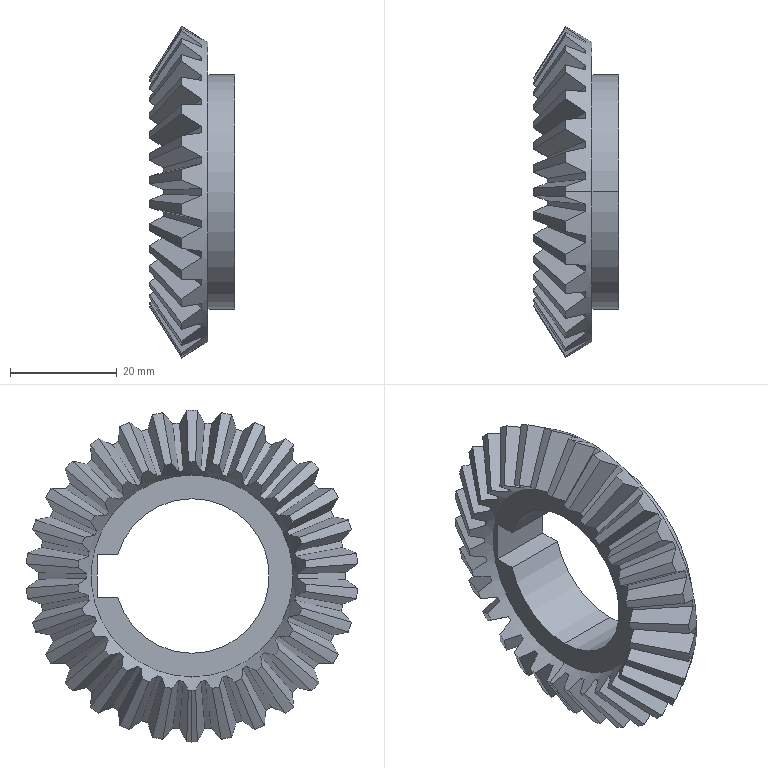Part | SolidWorks | features BlendCut 1, CirPattern 1, ICE 1, Revolution 1 | 1 solid | 136 faces | box 16 x 62.135 x 62.3 mm | volume 17909 mm3 | plane 96 | cone 35 | cylinder 5 | commonest cylinder face diameters 29 x3 44 x2